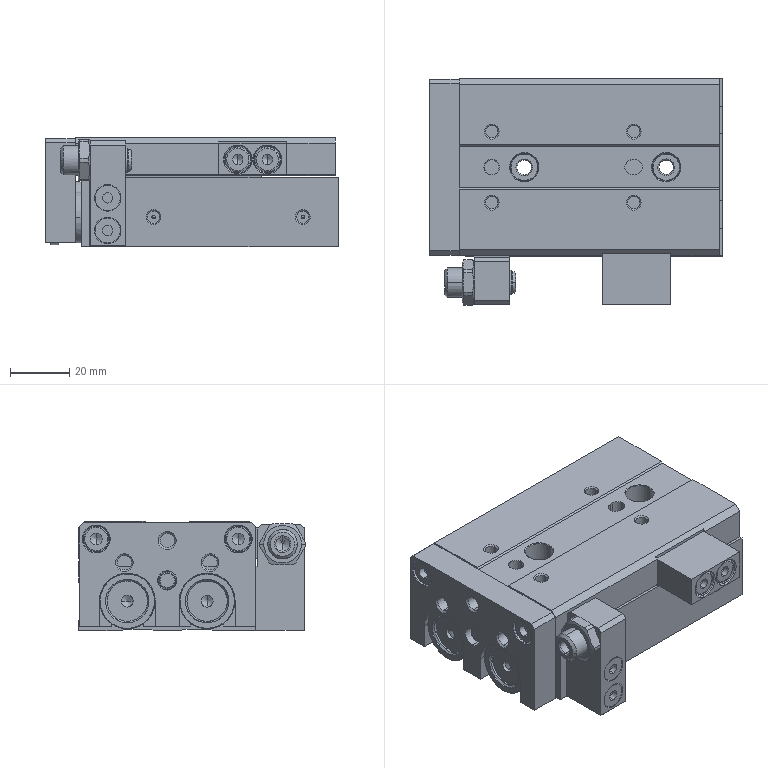Part | SolidWorks | 3 solids | 565 faces | box 99 x 76.75 x 37 mm | volume 182069 mm3 | plane 240 | cylinder 197 | cone 114 | spline 14 | commonest cylinder face diameters 4.134 x28 9 x20 8.5 x12 4 x11 4.917 x10 5 x10